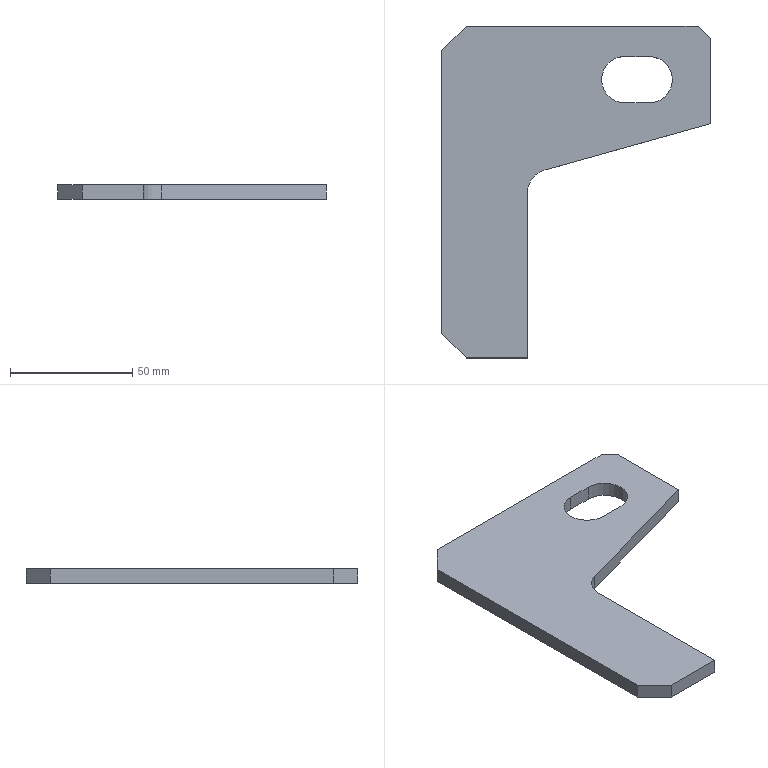Part | STEP file | 筋Plate-150×75-5 | 1 solid | 17 faces | box 110 x 136 x 6 mm | volume 47835 mm3 | plane 13 | cylinder 4 | commonest cylinder face diameters 19 x3 20 x1
STEP:
#1=CARTESIAN_POINT('',(0.,0.,0.));
#2=DIRECTION('',(0.,0.,1.));
#3=DIRECTION('',(1.,0.,0.));
#4=AXIS2_PLACEMENT_3D('',#1,#2,#3);
#5=CARTESIAN_POINT('',(20.,55.5,3.));
#6=VERTEX_POINT('',#5);
#7=CARTESIAN_POINT('',(20.,55.5,-3.));
#8=VERTEX_POINT('',#7);
#9=CARTESIAN_POINT('',(20.,55.5,-3.));
#10=DIRECTION('',(0.,0.,-1.));
#11=VECTOR('',#10,1.);
#12=LINE('',#9,#11);
#13=CARTESIAN_POINT('',(20.,46.,-3.));
#14=DIRECTION('',(0.,0.,-1.));
#15=DIRECTION('',(-1.,0.,0.));
#16=AXIS2_PLACEMENT_3D('',#13,#14,#15);
#17=CYLINDRICAL_SURFACE('',#16,9.5);
#18=CARTESIAN_POINT('',(1.571,0.));
#19=DIRECTION('',(0.,1.));
#20=VECTOR('',#19,1.);
#21=LINE('',#18,#20);
#22=(GEOMETRIC_REPRESENTATION_CONTEXT(2)PARAMETRIC_REPRESENTATION_CONTEXT()REPRESENTATION_CONTEXT('',''));
#23=DEFINITIONAL_REPRESENTATION('',(#21),#22);
#24=PCURVE('',#17,#23);
#25=CARTESIAN_POINT('',(20.,55.5,-3.));
#26=DIRECTION('',(0.,1.,0.));
#27=DIRECTION('',(0.,0.,1.));
#28=AXIS2_PLACEMENT_3D('',#25,#26,#27);
#29=PLANE('',#28);
#30=CARTESIAN_POINT('',(0.,0.));
#31=DIRECTION('',(-1.,0.));
#32=VECTOR('',#31,1.);
#33=LINE('',#30,#32);
#34=(GEOMETRIC_REPRESENTATION_CONTEXT(2)PARAMETRIC_REPRESENTATION_CONTEXT()REPRESENTATION_CONTEXT('',''));
#35=DEFINITIONAL_REPRESENTATION('',(#33),#34);
#36=PCURVE('',#29,#35);
#37=SURFACE_CURVE('',#12,(#24,#36),.PCURVE_S1.);
#38=EDGE_CURVE('',#6,#8,#37,.T.);
#39=ORIENTED_EDGE('',*,*,#38,.T.);
#40=CARTESIAN_POINT('',(10.5,46.,-3.));
#41=VERTEX_POINT('',#40);
#42=CARTESIAN_POINT('',(20.,46.,-3.));
#43=DIRECTION('',(0.,0.,-1.));
#44=DIRECTION('',(-1.,0.,0.));
#45=AXIS2_PLACEMENT_3D('',#42,#43,#44);
#46=CIRCLE('',#45,9.5);
#47=CARTESIAN_POINT('',(0.,0.));
#48=DIRECTION('',(1.,0.));
#49=VECTOR('',#48,1.);
#50=LINE('',#47,#49);
#51=(GEOMETRIC_REPRESENTATION_CONTEXT(2)PARAMETRIC_REPRESENTATION_CONTEXT()REPRESENTATION_CONTEXT('',''));
#52=DEFINITIONAL_REPRESENTATION('',(#50),#51);
#53=PCURVE('',#17,#52);
#54=CARTESIAN_POINT('',(0.,0.,-3.));
#55=DIRECTION('',(0.,0.,1.));
#56=DIRECTION('',(1.,0.,0.));
#57=AXIS2_PLACEMENT_3D('',#54,#55,#56);
#58=PLANE('',#57);
#59=CARTESIAN_POINT('',(10.5,46.));
#60=CARTESIAN_POINT('',(10.5,62.454));
#61=CARTESIAN_POINT('',(24.75,54.227));
#62=CARTESIAN_POINT('',(39.,46.));
#63=CARTESIAN_POINT('',(24.75,37.773));
#64=CARTESIAN_POINT('',(10.5,29.546));
#65=CARTESIAN_POINT('',(10.5,46.));
#66=(BOUNDED_CURVE()B_SPLINE_CURVE(2,(#59,#60,#61,#62,#63,#64,#65),.UNSPECIFIED.,.T.,.F.)B_SPLINE_CURVE_WITH_KNOTS((1,2,2,2,2,1),(-2.094,0.,2.094,4.189,6.283,8.378),.UNSPECIFIED.)CURVE()GEOMETRIC_REPRESENTATION_ITEM()RATIONAL_B_SPLINE_CURVE((1.,0.5,1.,0.5,1.,0.5,1.))REPRESENTATION_ITEM(''));
#67=(GEOMETRIC_REPRESENTATION_CONTEXT(2)PARAMETRIC_REPRESENTATION_CONTEXT()REPRESENTATION_CONTEXT('',''));
#68=DEFINITIONAL_REPRESENTATION('',(#66),#67);
#69=PCURVE('',#58,#68);
#70=SURFACE_CURVE('',#46,(#53,#69),.PCURVE_S1.);
#71=EDGE_CURVE('',#41,#8,#70,.T.);
#72=ORIENTED_EDGE('',*,*,#71,.F.);
#73=CARTESIAN_POINT('',(10.5,46.,3.));
#74=VERTEX_POINT('',#73);
#75=CARTESIAN_POINT('',(10.5,46.,-3.));
#76=DIRECTION('',(0.,0.,-1.));
#77=VECTOR('',#76,1.);
#78=LINE('',#75,#77);
#79=CARTESIAN_POINT('',(0.,0.));
#80=DIRECTION('',(0.,1.));
#81=VECTOR('',#80,1.);
#82=LINE('',#79,#81);
#83=(GEOMETRIC_REPRESENTATION_CONTEXT(2)PARAMETRIC_REPRESENTATION_CONTEXT()REPRESENTATION_CONTEXT('',''));
#84=DEFINITIONAL_REPRESENTATION('',(#82),#83);
#85=PCURVE('',#17,#84);
#86=CARTESIAN_POINT('',(20.,46.,-3.));
#87=DIRECTION('',(0.,0.,-1.));
#88=DIRECTION('',(-1.,0.,0.));
#89=AXIS2_PLACEMENT_3D('',#86,#87,#88);
#90=CYLINDRICAL_SURFACE('',#89,9.5);
#91=CARTESIAN_POINT('',(6.283,0.));
#92=DIRECTION('',(0.,1.));
#93=VECTOR('',#92,1.);
#94=LINE('',#91,#93);
#95=(GEOMETRIC_REPRESENTATION_CONTEXT(2)PARAMETRIC_REPRESENTATION_CONTEXT()REPRESENTATION_CONTEXT('',''));
#96=DEFINITIONAL_REPRESENTATION('',(#94),#95);
#97=PCURVE('',#90,#96);
#98=SURFACE_CURVE('',#78,(#85,#97),.PCURVE_S1.);
#99=EDGE_CURVE('',#74,#41,#98,.T.);
#100=ORIENTED_EDGE('',*,*,#99,.F.);
#101=CARTESIAN_POINT('',(20.,46.,3.));
#102=DIRECTION('',(0.,0.,1.));
#103=DIRECTION('',(1.,0.,0.));
#104=AXIS2_PLACEMENT_3D('',#101,#102,#103);
#105=CIRCLE('',#104,9.5);
#106=CARTESIAN_POINT('',(3.142,-6.));
#107=DIRECTION('',(-1.,0.));
#108=VECTOR('',#107,1.);
#109=LINE('',#106,#108);
#110=(GEOMETRIC_REPRESENTATION_CONTEXT(2)PARAMETRIC_REPRESENTATION_CONTEXT()REPRESENTATION_CONTEXT('',''));
#111=DEFINITIONAL_REPRESENTATION('',(#109),#110);
#112=PCURVE('',#17,#111);
#113=CARTESIAN_POINT('',(0.,0.,3.));
#114=DIRECTION('',(0.,0.,1.));
#115=DIRECTION('',(1.,0.,0.));
#116=AXIS2_PLACEMENT_3D('',#113,#114,#115);
#117=PLANE('',#116);
#118=CARTESIAN_POINT('',(20.,46.));
#119=DIRECTION('',(1.,0.));
#120=AXIS2_PLACEMENT_2D('',#118,#119);
#121=CIRCLE('',#120,9.5);
#122=(GEOMETRIC_REPRESENTATION_CONTEXT(2)PARAMETRIC_REPRESENTATION_CONTEXT()REPRESENTATION_CONTEXT('',''));
#123=DEFINITIONAL_REPRESENTATION('',(#121),#122);
#124=PCURVE('',#117,#123);
#125=SURFACE_CURVE('',#105,(#112,#124),.PCURVE_S1.);
#126=EDGE_CURVE('',#6,#74,#125,.T.);
#127=ORIENTED_EDGE('',*,*,#126,.F.);
#128=EDGE_LOOP('',(#39,#72,#100,#127));
#129=FACE_BOUND('',#128,.F.);
#130=ADVANCED_FACE('',(#129),#17,.F.);
#131=CARTESIAN_POINT('',(-45.,68.,-3.));
#132=VERTEX_POINT('',#131);
#133=CARTESIAN_POINT('',(50.,68.,-3.));
#134=VERTEX_POINT('',#133);
#135=CARTESIAN_POINT('',(0.,68.,-3.));
#136=DIRECTION('',(1.,0.,0.));
#137=VECTOR('',#136,1.);
#138=LINE('',#135,#137);
#139=CARTESIAN_POINT('',(0.,68.));
#140=DIRECTION('',(1.,0.));
#141=VECTOR('',#140,1.);
#142=LINE('',#139,#141);
#143=(GEOMETRIC_REPRESENTATION_CONTEXT(2)PARAMETRIC_REPRESENTATION_CONTEXT()REPRESENTATION_CONTEXT('',''));
#144=DEFINITIONAL_REPRESENTATION('',(#142),#143);
#145=PCURVE('',#58,#144);
#146=CARTESIAN_POINT('',(0.,68.,3.));
#147=DIRECTION('',(0.,1.,0.));
#148=DIRECTION('',(0.,0.,1.));
#149=AXIS2_PLACEMENT_3D('',#146,#147,#148);
#150=PLANE('',#149);
#151=CARTESIAN_POINT('',(-6.,0.));
#152=DIRECTION('',(0.,1.));
#153=VECTOR('',#152,1.);
#154=LINE('',#151,#153);
#155=(GEOMETRIC_REPRESENTATION_CONTEXT(2)PARAMETRIC_REPRESENTATION_CONTEXT()REPRESENTATION_CONTEXT('',''));
#156=DEFINITIONAL_REPRESENTATION('',(#154),#155);
#157=PCURVE('',#150,#156);
#158=SURFACE_CURVE('',#138,(#145,#157),.PCURVE_S1.);
#159=EDGE_CURVE('',#132,#134,#158,.T.);
#160=ORIENTED_EDGE('',*,*,#159,.T.);
#161=CARTESIAN_POINT('',(55.,63.,-3.));
#162=VERTEX_POINT('',#161);
#163=CARTESIAN_POINT('',(50.,68.,-3.));
#164=DIRECTION('',(0.7071,-0.7071,0.));
#165=VECTOR('',#164,1.);
#166=LINE('',#163,#165);
#167=CARTESIAN_POINT('',(50.,68.));
#168=DIRECTION('',(0.7071,-0.7071));
#169=VECTOR('',#168,1.);
#170=LINE('',#167,#169);
#171=(GEOMETRIC_REPRESENTATION_CONTEXT(2)PARAMETRIC_REPRESENTATION_CONTEXT()REPRESENTATION_CONTEXT('',''));
#172=DEFINITIONAL_REPRESENTATION('',(#170),#171);
#173=PCURVE('',#58,#172);
#174=CARTESIAN_POINT('',(50.,68.,3.));
#175=DIRECTION('',(-0.7071,-0.7071,0.));
#176=DIRECTION('',(0.,0.,-1.));
#177=AXIS2_PLACEMENT_3D('',#174,#175,#176);
#178=PLANE('',#177);
#179=CARTESIAN_POINT('',(6.,0.));
#180=DIRECTION('',(0.,1.));
#181=VECTOR('',#180,1.);
#182=LINE('',#179,#181);
#183=(GEOMETRIC_REPRESENTATION_CONTEXT(2)PARAMETRIC_REPRESENTATION_CONTEXT()REPRESENTATION_CONTEXT('',''));
#184=DEFINITIONAL_REPRESENTATION('',(#182),#183);
#185=PCURVE('',#178,#184);
#186=SURFACE_CURVE('',#166,(#173,#185),.PCURVE_S1.);
#187=EDGE_CURVE('',#134,#162,#186,.T.);
#188=ORIENTED_EDGE('',*,*,#187,.T.);
#189=CARTESIAN_POINT('',(55.,28.,-3.));
#190=VERTEX_POINT('',#189);
#191=CARTESIAN_POINT('',(55.,0.,-3.));
#192=DIRECTION('',(0.,-1.,0.));
#193=VECTOR('',#192,1.);
#194=LINE('',#191,#193);
#195=CARTESIAN_POINT('',(55.,0.));
#196=DIRECTION('',(0.,-1.));
#197=VECTOR('',#196,1.);
#198=LINE('',#195,#197);
#199=(GEOMETRIC_REPRESENTATION_CONTEXT(2)PARAMETRIC_REPRESENTATION_CONTEXT()REPRESENTATION_CONTEXT('',''));
#200=DEFINITIONAL_REPRESENTATION('',(#198),#199);
#201=PCURVE('',#58,#200);
#202=CARTESIAN_POINT('',(55.,0.,3.));
#203=DIRECTION('',(1.,0.,0.));
#204=DIRECTION('',(0.,1.,0.));
#205=AXIS2_PLACEMENT_3D('',#202,#203,#204);
#206=PLANE('',#205);
#207=CARTESIAN_POINT('',(0.,-6.));
#208=DIRECTION('',(-1.,0.));
#209=VECTOR('',#208,1.);
#210=LINE('',#207,#209);
#211=(GEOMETRIC_REPRESENTATION_CONTEXT(2)PARAMETRIC_REPRESENTATION_CONTEXT()REPRESENTATION_CONTEXT('',''));
#212=DEFINITIONAL_REPRESENTATION('',(#210),#211);
#213=PCURVE('',#206,#212);
#214=SURFACE_CURVE('',#194,(#201,#213),.PCURVE_S1.);
#215=EDGE_CURVE('',#162,#190,#214,.T.);
#216=ORIENTED_EDGE('',*,*,#215,.T.);
#217=CARTESIAN_POINT('',(-12.696,9.045,-3.));
#218=VERTEX_POINT('',#217);
#219=CARTESIAN_POINT('',(55.,28.,-3.));
#220=DIRECTION('',(-0.963,-0.2696,0.));
#221=VECTOR('',#220,1.);
#222=LINE('',#219,#221);
#223=CARTESIAN_POINT('',(55.,28.));
#224=DIRECTION('',(-0.963,-0.2696));
#225=VECTOR('',#224,1.);
#226=LINE('',#223,#225);
#227=(GEOMETRIC_REPRESENTATION_CONTEXT(2)PARAMETRIC_REPRESENTATION_CONTEXT()REPRESENTATION_CONTEXT('',''));
#228=DEFINITIONAL_REPRESENTATION('',(#226),#227);
#229=PCURVE('',#58,#228);
#230=CARTESIAN_POINT('',(55.,28.,-3.));
#231=DIRECTION('',(-0.2696,0.963,0.));
#232=DIRECTION('',(-0.963,-0.2696,0.));
#233=AXIS2_PLACEMENT_3D('',#230,#231,#232);
#234=PLANE('',#233);
#235=CARTESIAN_POINT('',(0.,0.));
#236=DIRECTION('',(1.,0.));
#237=VECTOR('',#236,1.);
#238=LINE('',#235,#237);
#239=(GEOMETRIC_REPRESENTATION_CONTEXT(2)PARAMETRIC_REPRESENTATION_CONTEXT()REPRESENTATION_CONTEXT('',''));
#240=DEFINITIONAL_REPRESENTATION('',(#238),#239);
#241=PCURVE('',#234,#240);
#242=SURFACE_CURVE('',#222,(#229,#241),.PCURVE_S1.);
#243=EDGE_CURVE('',#190,#218,#242,.T.);
#244=ORIENTED_EDGE('',*,*,#243,.T.);
#245=CARTESIAN_POINT('',(-20.,-0.5846,-3.));
#246=VERTEX_POINT('',#245);
#247=CARTESIAN_POINT('',(-10.,-0.5846,-3.));
#248=DIRECTION('',(0.,0.,1.));
#249=DIRECTION('',(1.,0.,0.));
#250=AXIS2_PLACEMENT_3D('',#247,#248,#249);
#251=CIRCLE('',#250,10.);
#252=CARTESIAN_POINT('',(-10.,-0.5846));
#253=DIRECTION('',(1.,0.));
#254=AXIS2_PLACEMENT_2D('',#252,#253);
#255=CIRCLE('',#254,10.);
#256=(GEOMETRIC_REPRESENTATION_CONTEXT(2)PARAMETRIC_REPRESENTATION_CONTEXT()REPRESENTATION_CONTEXT('',''));
#257=DEFINITIONAL_REPRESENTATION('',(#255),#256);
#258=PCURVE('',#58,#257);
#259=CARTESIAN_POINT('',(-10.,-0.5846,-3.));
#260=DIRECTION('',(0.,0.,-1.));
#261=DIRECTION('',(-1.,0.,0.));
#262=AXIS2_PLACEMENT_3D('',#259,#260,#261);
#263=CYLINDRICAL_SURFACE('',#262,10.);
#264=CARTESIAN_POINT('',(3.142,0.));
#265=DIRECTION('',(-1.,0.));
#266=VECTOR('',#265,1.);
#267=LINE('',#264,#266);
#268=(GEOMETRIC_REPRESENTATION_CONTEXT(2)PARAMETRIC_REPRESENTATION_CONTEXT()REPRESENTATION_CONTEXT('',''));
#269=DEFINITIONAL_REPRESENTATION('',(#267),#268);
#270=PCURVE('',#263,#269);
#271=SURFACE_CURVE('',#251,(#258,#270),.PCURVE_S1.);
#272=EDGE_CURVE('',#218,#246,#271,.T.);
#273=ORIENTED_EDGE('',*,*,#272,.T.);
#274=CARTESIAN_POINT('',(-20.,-68.,-3.));
#275=VERTEX_POINT('',#274);
#276=CARTESIAN_POINT('',(-20.,-68.,-3.));
#277=DIRECTION('',(0.,-1.,0.));
#278=VECTOR('',#277,1.);
#279=LINE('',#276,#278);
#280=CARTESIAN_POINT('',(-20.,-68.));
#281=DIRECTION('',(0.,-1.));
#282=VECTOR('',#281,1.);
#283=LINE('',#280,#282);
#284=(GEOMETRIC_REPRESENTATION_CONTEXT(2)PARAMETRIC_REPRESENTATION_CONTEXT()REPRESENTATION_CONTEXT('',''));
#285=DEFINITIONAL_REPRESENTATION('',(#283),#284);
#286=PCURVE('',#58,#285);
#287=CARTESIAN_POINT('',(-20.,-68.,-3.));
#288=DIRECTION('',(-1.,0.,0.));
#289=DIRECTION('',(0.,0.,1.));
#290=AXIS2_PLACEMENT_3D('',#287,#288,#289);
#291=PLANE('',#290);
#292=CARTESIAN_POINT('',(0.,0.));
#293=DIRECTION('',(0.,-1.));
#294=VECTOR('',#293,1.);
#295=LINE('',#292,#294);
#296=(GEOMETRIC_REPRESENTATION_CONTEXT(2)PARAMETRIC_REPRESENTATION_CONTEXT()REPRESENTATION_CONTEXT('',''));
#297=DEFINITIONAL_REPRESENTATION('',(#295),#296);
#298=PCURVE('',#291,#297);
#299=SURFACE_CURVE('',#279,(#286,#298),.PCURVE_S1.);
#300=EDGE_CURVE('',#246,#275,#299,.T.);
#301=ORIENTED_EDGE('',*,*,#300,.T.);
#302=CARTESIAN_POINT('',(-45.,-68.,-3.));
#303=VERTEX_POINT('',#302);
#304=CARTESIAN_POINT('',(0.,-68.,-3.));
#305=DIRECTION('',(1.,0.,0.));
#306=VECTOR('',#305,1.);
#307=LINE('',#304,#306);
#308=CARTESIAN_POINT('',(0.,-68.));
#309=DIRECTION('',(1.,0.));
#310=VECTOR('',#309,1.);
#311=LINE('',#308,#310);
#312=(GEOMETRIC_REPRESENTATION_CONTEXT(2)PARAMETRIC_REPRESENTATION_CONTEXT()REPRESENTATION_CONTEXT('',''));
#313=DEFINITIONAL_REPRESENTATION('',(#311),#312);
#314=PCURVE('',#58,#313);
#315=CARTESIAN_POINT('',(0.,-68.,3.));
#316=DIRECTION('',(0.,1.,0.));
#317=DIRECTION('',(0.,0.,1.));
#318=AXIS2_PLACEMENT_3D('',#315,#316,#317);
#319=PLANE('',#318);
#320=CARTESIAN_POINT('',(-6.,0.));
#321=DIRECTION('',(0.,1.));
#322=VECTOR('',#321,1.);
#323=LINE('',#320,#322);
#324=(GEOMETRIC_REPRESENTATION_CONTEXT(2)PARAMETRIC_REPRESENTATION_CONTEXT()REPRESENTATION_CONTEXT('',''));
#325=DEFINITIONAL_REPRESENTATION('',(#323),#324);
#326=PCURVE('',#319,#325);
#327=SURFACE_CURVE('',#307,(#314,#326),.PCURVE_S1.);
#328=EDGE_CURVE('',#303,#275,#327,.T.);
#329=ORIENTED_EDGE('',*,*,#328,.F.);
#330=CARTESIAN_POINT('',(-55.,-58.,-3.));
#331=VERTEX_POINT('',#330);
#332=CARTESIAN_POINT('',(-45.,-68.,-3.));
#333=DIRECTION('',(-0.7071,0.7071,0.));
#334=VECTOR('',#333,1.);
#335=LINE('',#332,#334);
#336=CARTESIAN_POINT('',(-45.,-68.));
#337=DIRECTION('',(-0.7071,0.7071));
#338=VECTOR('',#337,1.);
#339=LINE('',#336,#338);
#340=(GEOMETRIC_REPRESENTATION_CONTEXT(2)PARAMETRIC_REPRESENTATION_CONTEXT()REPRESENTATION_CONTEXT('',''));
#341=DEFINITIONAL_REPRESENTATION('',(#339),#340);
#342=PCURVE('',#58,#341);
#343=CARTESIAN_POINT('',(-45.,-68.,3.));
#344=DIRECTION('',(0.7071,0.7071,0.));
#345=DIRECTION('',(0.,0.,-1.));
#346=AXIS2_PLACEMENT_3D('',#343,#344,#345);
#347=PLANE('',#346);
#348=CARTESIAN_POINT('',(6.,0.));
#349=DIRECTION('',(0.,1.));
#350=VECTOR('',#349,1.);
#351=LINE('',#348,#350);
#352=(GEOMETRIC_REPRESENTATION_CONTEXT(2)PARAMETRIC_REPRESENTATION_CONTEXT()REPRESENTATION_CONTEXT('',''));
#353=DEFINITIONAL_REPRESENTATION('',(#351),#352);
#354=PCURVE('',#347,#353);
#355=SURFACE_CURVE('',#335,(#342,#354),.PCURVE_S1.);
#356=EDGE_CURVE('',#303,#331,#355,.T.);
#357=ORIENTED_EDGE('',*,*,#356,.T.);
#358=CARTESIAN_POINT('',(-55.,58.,-3.));
#359=VERTEX_POINT('',#358);
#360=CARTESIAN_POINT('',(-55.,0.,-3.));
#361=DIRECTION('',(0.,-1.,0.));
#362=VECTOR('',#361,1.);
#363=LINE('',#360,#362);
#364=CARTESIAN_POINT('',(-55.,0.));
#365=DIRECTION('',(0.,-1.));
#366=VECTOR('',#365,1.);
#367=LINE('',#364,#366);
#368=(GEOMETRIC_REPRESENTATION_CONTEXT(2)PARAMETRIC_REPRESENTATION_CONTEXT()REPRESENTATION_CONTEXT('',''));
#369=DEFINITIONAL_REPRESENTATION('',(#367),#368);
#370=PCURVE('',#58,#369);
#371=CARTESIAN_POINT('',(-55.,0.,3.));
#372=DIRECTION('',(1.,0.,0.));
#373=DIRECTION('',(0.,1.,0.));
#374=AXIS2_PLACEMENT_3D('',#371,#372,#373);
#375=PLANE('',#374);
#376=CARTESIAN_POINT('',(0.,-6.));
#377=DIRECTION('',(-1.,0.));
#378=VECTOR('',#377,1.);
#379=LINE('',#376,#378);
#380=(GEOMETRIC_REPRESENTATION_CONTEXT(2)PARAMETRIC_REPRESENTATION_CONTEXT()REPRESENTATION_CONTEXT('',''));
#381=DEFINITIONAL_REPRESENTATION('',(#379),#380);
#382=PCURVE('',#375,#381);
#383=SURFACE_CURVE('',#363,(#370,#382),.PCURVE_S1.);
#384=EDGE_CURVE('',#359,#331,#383,.T.);
#385=ORIENTED_EDGE('',*,*,#384,.F.);
#386=CARTESIAN_POINT('',(-55.,58.,-3.));
#387=DIRECTION('',(0.7071,0.7071,0.));
#388=VECTOR('',#387,1.);
#389=LINE('',#386,#388);
#390=CARTESIAN_POINT('',(-55.,58.));
#391=DIRECTION('',(0.7071,0.7071));
#392=VECTOR('',#391,1.);
#393=LINE('',#390,#392);
#394=(GEOMETRIC_REPRESENTATION_CONTEXT(2)PARAMETRIC_REPRESENTATION_CONTEXT()REPRESENTATION_CONTEXT('',''));
#395=DEFINITIONAL_REPRESENTATION('',(#393),#394);
#396=PCURVE('',#58,#395);
#397=CARTESIAN_POINT('',(-55.,58.,3.));
#398=DIRECTION('',(-0.7071,0.7071,0.));
#399=DIRECTION('',(0.,0.,1.));
#400=AXIS2_PLACEMENT_3D('',#397,#398,#399);
#401=PLANE('',#400);
#402=CARTESIAN_POINT('',(-6.,0.));
#403=DIRECTION('',(0.,1.));
#404=VECTOR('',#403,1.);
#405=LINE('',#402,#404);
#406=(GEOMETRIC_REPRESENTATION_CONTEXT(2)PARAMETRIC_REPRESENTATION_CONTEXT()REPRESENTATION_CONTEXT('',''));
#407=DEFINITIONAL_REPRESENTATION('',(#405),#406);
#408=PCURVE('',#401,#407);
#409=SURFACE_CURVE('',#389,(#396,#408),.PCURVE_S1.);
#410=EDGE_CURVE('',#359,#132,#409,.T.);
#411=ORIENTED_EDGE('',*,*,#410,.T.);
#412=EDGE_LOOP('',(#160,#188,#216,#244,#273,#301,#329,#357,#385,#411));
#413=FACE_BOUND('',#412,.T.);
#414=CARTESIAN_POINT('',(30.,55.5,-3.));
#415=VERTEX_POINT('',#414);
#416=CARTESIAN_POINT('',(30.,36.5,-3.));
#417=VERTEX_POINT('',#416);
#418=CARTESIAN_POINT('',(30.,46.,-3.));
#419=DIRECTION('',(0.,0.,-1.));
#420=DIRECTION('',(-1.,0.,0.));
#421=AXIS2_PLACEMENT_3D('',#418,#419,#420);
#422=CIRCLE('',#421,9.5);
#423=CARTESIAN_POINT('',(20.5,46.));
#424=CARTESIAN_POINT('',(20.5,62.454));
#425=CARTESIAN_POINT('',(34.75,54.227));
#426=CARTESIAN_POINT('',(49.,46.));
#427=CARTESIAN_POINT('',(34.75,37.773));
#428=CARTESIAN_POINT('',(20.5,29.546));
#429=CARTESIAN_POINT('',(20.5,46.));
#430=(BOUNDED_CURVE()B_SPLINE_CURVE(2,(#423,#424,#425,#426,#427,#428,#429),.UNSPECIFIED.,.T.,.F.)B_SPLINE_CURVE_WITH_KNOTS((1,2,2,2,2,1),(-2.094,0.,2.094,4.189,6.283,8.378),.UNSPECIFIED.)CURVE()GEOMETRIC_REPRESENTATION_ITEM()RATIONAL_B_SPLINE_CURVE((1.,0.5,1.,0.5,1.,0.5,1.))REPRESENTATION_ITEM(''));
#431=(GEOMETRIC_REPRESENTATION_CONTEXT(2)PARAMETRIC_REPRESENTATION_CONTEXT()REPRESENTATION_CONTEXT('',''));
#432=DEFINITIONAL_REPRESENTATION('',(#430),#431);
#433=PCURVE('',#58,#432);
#434=CARTESIAN_POINT('',(30.,46.,-3.));
#435=DIRECTION('',(0.,0.,-1.));
#436=DIRECTION('',(-1.,0.,0.));
#437=AXIS2_PLACEMENT_3D('',#434,#435,#436);
#438=CYLINDRICAL_SURFACE('',#437,9.5);
#439=CARTESIAN_POINT('',(0.,0.));
#440=DIRECTION('',(1.,0.));
#441=VECTOR('',#440,1.);
#442=LINE('',#439,#441);
#443=(GEOMETRIC_REPRESENTATION_CONTEXT(2)PARAMETRIC_REPRESENTATION_CONTEXT()REPRESENTATION_CONTEXT('',''));
#444=DEFINITIONAL_REPRESENTATION('',(#442),#443);
#445=PCURVE('',#438,#444);
#446=SURFACE_CURVE('',#422,(#433,#445),.PCURVE_S1.);
#447=EDGE_CURVE('',#415,#417,#446,.T.);
#448=ORIENTED_EDGE('',*,*,#447,.F.);
#449=CARTESIAN_POINT('',(20.,55.5,-3.));
#450=DIRECTION('',(1.,0.,0.));
#451=VECTOR('',#450,1.);
#452=LINE('',#449,#451);
#453=CARTESIAN_POINT('',(20.,55.5));
#454=DIRECTION('',(1.,0.));
#455=VECTOR('',#454,1.);
#456=LINE('',#453,#455);
#457=(GEOMETRIC_REPRESENTATION_CONTEXT(2)PARAMETRIC_REPRESENTATION_CONTEXT()REPRESENTATION_CONTEXT('',''));
#458=DEFINITIONAL_REPRESENTATION('',(#456),#457);
#459=PCURVE('',#58,#458);
#460=CARTESIAN_POINT('',(0.,0.));
#461=DIRECTION('',(0.,1.));
#462=VECTOR('',#461,1.);
#463=LINE('',#460,#462);
#464=(GEOMETRIC_REPRESENTATION_CONTEXT(2)PARAMETRIC_REPRESENTATION_CONTEXT()REPRESENTATION_CONTEXT('',''));
#465=DEFINITIONAL_REPRESENTATION('',(#463),#464);
#466=PCURVE('',#29,#465);
#467=SURFACE_CURVE('',#452,(#459,#466),.PCURVE_S1.);
#468=EDGE_CURVE('',#8,#415,#467,.T.);
#469=ORIENTED_EDGE('',*,*,#468,.F.);
#470=ORIENTED_EDGE('',*,*,#71,.F.);
#471=CARTESIAN_POINT('',(20.,36.5,-3.));
#472=VERTEX_POINT('',#471);
#473=CARTESIAN_POINT('',(20.,46.,-3.));
#474=DIRECTION('',(0.,0.,-1.));
#475=DIRECTION('',(-1.,0.,0.));
#476=AXIS2_PLACEMENT_3D('',#473,#474,#475);
#477=CIRCLE('',#476,9.5);
#478=CARTESIAN_POINT('',(10.5,46.));
#479=CARTESIAN_POINT('',(10.5,62.454));
#480=CARTESIAN_POINT('',(24.75,54.227));
#481=CARTESIAN_POINT('',(39.,46.));
#482=CARTESIAN_POINT('',(24.75,37.773));
#483=CARTESIAN_POINT('',(10.5,29.546));
#484=CARTESIAN_POINT('',(10.5,46.));
#485=(BOUNDED_CURVE()B_SPLINE_CURVE(2,(#478,#479,#480,#481,#482,#483,#484),.UNSPECIFIED.,.T.,.F.)B_SPLINE_CURVE_WITH_KNOTS((1,2,2,2,2,1),(-2.094,0.,2.094,4.189,6.283,8.378),.UNSPECIFIED.)CURVE()GEOMETRIC_REPRESENTATION_ITEM()RATIONAL_B_SPLINE_CURVE((1.,0.5,1.,0.5,1.,0.5,1.))REPRESENTATION_ITEM(''));
#486=(GEOMETRIC_REPRESENTATION_CONTEXT(2)PARAMETRIC_REPRESENTATION_CONTEXT()REPRESENTATION_CONTEXT('',''));
#487=DEFINITIONAL_REPRESENTATION('',(#485),#486);
#488=PCURVE('',#58,#487);
#489=CARTESIAN_POINT('',(0.,0.));
#490=DIRECTION('',(1.,0.));
#491=VECTOR('',#490,1.);
#492=LINE('',#489,#491);
#493=(GEOMETRIC_REPRESENTATION_CONTEXT(2)PARAMETRIC_REPRESENTATION_CONTEXT()REPRESENTATION_CONTEXT('',''));
#494=DEFINITIONAL_REPRESENTATION('',(#492),#493);
#495=PCURVE('',#90,#494);
#496=SURFACE_CURVE('',#477,(#488,#495),.PCURVE_S1.);
#497=EDGE_CURVE('',#472,#41,#496,.T.);
#498=ORIENTED_EDGE('',*,*,#497,.F.);
#499=CARTESIAN_POINT('',(20.,36.5,-3.));
#500=DIRECTION('',(1.,0.,0.));
#501=VECTOR('',#500,1.);
#502=LINE('',#499,#501);
#503=CARTESIAN_POINT('',(20.,36.5));
#504=DIRECTION('',(1.,0.));
#505=VECTOR('',#504,1.);
#506=LINE('',#503,#505);
#507=(GEOMETRIC_REPRESENTATION_CONTEXT(2)PARAMETRIC_REPRESENTATION_CONTEXT()REPRESENTATION_CONTEXT('',''));
#508=DEFINITIONAL_REPRESENTATION('',(#506),#507);
#509=PCURVE('',#58,#508);
#510=CARTESIAN_POINT('',(20.,36.5,-3.));
#511=DIRECTION('',(0.,-1.,0.));
#512=DIRECTION('',(0.,0.,-1.));
#513=AXIS2_PLACEMENT_3D('',#510,#511,#512);
#514=PLANE('',#513);
#515=CARTESIAN_POINT('',(0.,0.));
#516=DIRECTION('',(0.,1.));
#517=VECTOR('',#516,1.);
#518=LINE('',#515,#517);
#519=(GEOMETRIC_REPRESENTATION_CONTEXT(2)PARAMETRIC_REPRESENTATION_CONTEXT()REPRESENTATION_CONTEXT('',''));
#520=DEFINITIONAL_REPRESENTATION('',(#518),#519);
#521=PCURVE('',#514,#520);
#522=SURFACE_CURVE('',#502,(#509,#521),.PCURVE_S1.);
#523=EDGE_CURVE('',#472,#417,#522,.T.);
#524=ORIENTED_EDGE('',*,*,#523,.T.);
#525=EDGE_LOOP('',(#448,#469,#470,#498,#524));
#526=FACE_BOUND('',#525,.T.);
#527=ADVANCED_FACE('',(#413,#526),#58,.F.);
#528=ORIENTED_EDGE('',*,*,#215,.F.);
#529=CARTESIAN_POINT('',(55.,63.,3.));
#530=VERTEX_POINT('',#529);
#531=CARTESIAN_POINT('',(55.,63.,3.));
#532=DIRECTION('',(0.,0.,1.));
#533=VECTOR('',#532,1.);
#534=LINE('',#531,#533);
#535=CARTESIAN_POINT('',(63.,0.));
#536=DIRECTION('',(0.,1.));
#537=VECTOR('',#536,1.);
#538=LINE('',#535,#537);
#539=(GEOMETRIC_REPRESENTATION_CONTEXT(2)PARAMETRIC_REPRESENTATION_CONTEXT()REPRESENTATION_CONTEXT('',''));
#540=DEFINITIONAL_REPRESENTATION('',(#538),#539);
#541=PCURVE('',#206,#540);
#542=CARTESIAN_POINT('',(0.,7.071));
#543=DIRECTION('',(-1.,0.));
#544=VECTOR('',#543,1.);
#545=LINE('',#542,#544);
#546=(GEOMETRIC_REPRESENTATION_CONTEXT(2)PARAMETRIC_REPRESENTATION_CONTEXT()REPRESENTATION_CONTEXT('',''));
#547=DEFINITIONAL_REPRESENTATION('',(#545),#546);
#548=PCURVE('',#178,#547);
#549=SURFACE_CURVE('',#534,(#541,#548),.PCURVE_S1.);
#550=EDGE_CURVE('',#162,#530,#549,.T.);
#551=ORIENTED_EDGE('',*,*,#550,.T.);
#552=CARTESIAN_POINT('',(55.,28.,3.));
#553=VERTEX_POINT('',#552);
#554=CARTESIAN_POINT('',(55.,0.,3.));
#555=DIRECTION('',(0.,-1.,0.));
#556=VECTOR('',#555,1.);
#557=LINE('',#554,#556);
#558=CARTESIAN_POINT('',(0.,0.));
#559=DIRECTION('',(-1.,0.));
#560=VECTOR('',#559,1.);
#561=LINE('',#558,#560);
#562=(GEOMETRIC_REPRESENTATION_CONTEXT(2)PARAMETRIC_REPRESENTATION_CONTEXT()REPRESENTATION_CONTEXT('',''));
#563=DEFINITIONAL_REPRESENTATION('',(#561),#562);
#564=PCURVE('',#206,#563);
#565=CARTESIAN_POINT('',(55.,0.));
#566=DIRECTION('',(0.,-1.));
#567=VECTOR('',#566,1.);
#568=LINE('',#565,#567);
#569=(GEOMETRIC_REPRESENTATION_CONTEXT(2)PARAMETRIC_REPRESENTATION_CONTEXT()REPRESENTATION_CONTEXT('',''));
#570=DEFINITIONAL_REPRESENTATION('',(#568),#569);
#571=PCURVE('',#117,#570);
#572=SURFACE_CURVE('',#557,(#564,#571),.PCURVE_S1.);
#573=EDGE_CURVE('',#530,#553,#572,.T.);
#574=ORIENTED_EDGE('',*,*,#573,.T.);
#575=CARTESIAN_POINT('',(55.,28.,-3.));
#576=DIRECTION('',(0.,0.,1.));
#577=VECTOR('',#576,1.);
#578=LINE('',#575,#577);
#579=CARTESIAN_POINT('',(28.,-6.));
#580=DIRECTION('',(0.,1.));
#581=VECTOR('',#580,1.);
#582=LINE('',#579,#581);
#583=(GEOMETRIC_REPRESENTATION_CONTEXT(2)PARAMETRIC_REPRESENTATION_CONTEXT()REPRESENTATION_CONTEXT('',''));
#584=DEFINITIONAL_REPRESENTATION('',(#582),#583);
#585=PCURVE('',#206,#584);
#586=CARTESIAN_POINT('',(0.,0.));
#587=DIRECTION('',(0.,1.));
#588=VECTOR('',#587,1.);
#589=LINE('',#586,#588);
#590=(GEOMETRIC_REPRESENTATION_CONTEXT(2)PARAMETRIC_REPRESENTATION_CONTEXT()REPRESENTATION_CONTEXT('',''));
#591=DEFINITIONAL_REPRESENTATION('',(#589),#590);
#592=PCURVE('',#234,#591);
#593=SURFACE_CURVE('',#578,(#585,#592),.PCURVE_S1.);
#594=EDGE_CURVE('',#190,#553,#593,.T.);
#595=ORIENTED_EDGE('',*,*,#594,.F.);
#596=EDGE_LOOP('',(#528,#551,#574,#595));
#597=FACE_BOUND('',#596,.T.);
#598=ADVANCED_FACE('',(#597),#206,.T.);
#599=CARTESIAN_POINT('',(-45.,68.,3.));
#600=VERTEX_POINT('',#599);
#601=CARTESIAN_POINT('',(50.,68.,3.));
#602=VERTEX_POINT('',#601);
#603=CARTESIAN_POINT('',(0.,68.,3.));
#604=DIRECTION('',(1.,0.,0.));
#605=VECTOR('',#604,1.);
#606=LINE('',#603,#605);
#607=CARTESIAN_POINT('',(0.,0.));
#608=DIRECTION('',(0.,1.));
#609=VECTOR('',#608,1.);
#610=LINE('',#607,#609);
#611=(GEOMETRIC_REPRESENTATION_CONTEXT(2)PARAMETRIC_REPRESENTATION_CONTEXT()REPRESENTATION_CONTEXT('',''));
#612=DEFINITIONAL_REPRESENTATION('',(#610),#611);
#613=PCURVE('',#150,#612);
#614=CARTESIAN_POINT('',(0.,68.));
#615=DIRECTION('',(1.,0.));
#616=VECTOR('',#615,1.);
#617=LINE('',#614,#616);
#618=(GEOMETRIC_REPRESENTATION_CONTEXT(2)PARAMETRIC_REPRESENTATION_CONTEXT()REPRESENTATION_CONTEXT('',''));
#619=DEFINITIONAL_REPRESENTATION('',(#617),#618);
#620=PCURVE('',#117,#619);
#621=SURFACE_CURVE('',#606,(#613,#620),.PCURVE_S1.);
#622=EDGE_CURVE('',#600,#602,#621,.T.);
#623=ORIENTED_EDGE('',*,*,#622,.T.);
#624=CARTESIAN_POINT('',(50.,68.,3.));
#625=DIRECTION('',(0.,0.,-1.));
#626=VECTOR('',#625,1.);
#627=LINE('',#624,#626);
#628=CARTESIAN_POINT('',(0.,50.));
#629=DIRECTION('',(-1.,0.));
#630=VECTOR('',#629,1.);
#631=LINE('',#628,#630);
#632=(GEOMETRIC_REPRESENTATION_CONTEXT(2)PARAMETRIC_REPRESENTATION_CONTEXT()REPRESENTATION_CONTEXT('',''));
#633=DEFINITIONAL_REPRESENTATION('',(#631),#632);
#634=PCURVE('',#150,#633);
#635=CARTESIAN_POINT('',(0.,0.));
#636=DIRECTION('',(1.,0.));
#637=VECTOR('',#636,1.);
#638=LINE('',#635,#637);
#639=(GEOMETRIC_REPRESENTATION_CONTEXT(2)PARAMETRIC_REPRESENTATION_CONTEXT()REPRESENTATION_CONTEXT('',''));
#640=DEFINITIONAL_REPRESENTATION('',(#638),#639);
#641=PCURVE('',#178,#640);
#642=SURFACE_CURVE('',#627,(#634,#641),.PCURVE_S1.);
#643=EDGE_CURVE('',#602,#134,#642,.T.);
#644=ORIENTED_EDGE('',*,*,#643,.T.);
#645=ORIENTED_EDGE('',*,*,#159,.F.);
#646=CARTESIAN_POINT('',(-45.,68.,3.));
#647=DIRECTION('',(0.,0.,1.));
#648=VECTOR('',#647,1.);
#649=LINE('',#646,#648);
#650=CARTESIAN_POINT('',(0.,-45.));
#651=DIRECTION('',(1.,0.));
#652=VECTOR('',#651,1.);
#653=LINE('',#650,#652);
#654=(GEOMETRIC_REPRESENTATION_CONTEXT(2)PARAMETRIC_REPRESENTATION_CONTEXT()REPRESENTATION_CONTEXT('',''));
#655=DEFINITIONAL_REPRESENTATION('',(#653),#654);
#656=PCURVE('',#150,#655);
#657=CARTESIAN_POINT('',(0.,14.142));
#658=DIRECTION('',(1.,0.));
#659=VECTOR('',#658,1.);
#660=LINE('',#657,#659);
#661=(GEOMETRIC_REPRESENTATION_CONTEXT(2)PARAMETRIC_REPRESENTATION_CONTEXT()REPRESENTATION_CONTEXT('',''));
#662=DEFINITIONAL_REPRESENTATION('',(#660),#661);
#663=PCURVE('',#401,#662);
#664=SURFACE_CURVE('',#649,(#656,#663),.PCURVE_S1.);
#665=EDGE_CURVE('',#132,#600,#664,.T.);
#666=ORIENTED_EDGE('',*,*,#665,.T.);
#667=EDGE_LOOP('',(#623,#644,#645,#666));
#668=FACE_BOUND('',#667,.T.);
#669=ADVANCED_FACE('',(#668),#150,.T.);
#670=ORIENTED_EDGE('',*,*,#384,.T.);
#671=CARTESIAN_POINT('',(-55.,-58.,3.));
#672=VERTEX_POINT('',#671);
#673=CARTESIAN_POINT('',(-55.,-58.,3.));
#674=DIRECTION('',(0.,0.,1.));
#675=VECTOR('',#674,1.);
#676=LINE('',#673,#675);
#677=CARTESIAN_POINT('',(-58.,0.));
#678=DIRECTION('',(0.,1.));
#679=VECTOR('',#678,1.);
#680=LINE('',#677,#679);
#681=(GEOMETRIC_REPRESENTATION_CONTEXT(2)PARAMETRIC_REPRESENTATION_CONTEXT()REPRESENTATION_CONTEXT('',''));
#682=DEFINITIONAL_REPRESENTATION('',(#680),#681);
#683=PCURVE('',#375,#682);
#684=CARTESIAN_POINT('',(0.,14.142));
#685=DIRECTION('',(-1.,0.));
#686=VECTOR('',#685,1.);
#687=LINE('',#684,#686);
#688=(GEOMETRIC_REPRESENTATION_CONTEXT(2)PARAMETRIC_REPRESENTATION_CONTEXT()REPRESENTATION_CONTEXT('',''));
#689=DEFINITIONAL_REPRESENTATION('',(#687),#688);
#690=PCURVE('',#347,#689);
#691=SURFACE_CURVE('',#676,(#683,#690),.PCURVE_S1.);
#692=EDGE_CURVE('',#331,#672,#691,.T.);
#693=ORIENTED_EDGE('',*,*,#692,.T.);
#694=CARTESIAN_POINT('',(-55.,58.,3.));
#695=VERTEX_POINT('',#694);
#696=CARTESIAN_POINT('',(-55.,0.,3.));
#697=DIRECTION('',(0.,-1.,0.));
#698=VECTOR('',#697,1.);
#699=LINE('',#696,#698);
#700=CARTESIAN_POINT('',(0.,0.));
#701=DIRECTION('',(-1.,0.));
#702=VECTOR('',#701,1.);
#703=LINE('',#700,#702);
#704=(GEOMETRIC_REPRESENTATION_CONTEXT(2)PARAMETRIC_REPRESENTATION_CONTEXT()REPRESENTATION_CONTEXT('',''));
#705=DEFINITIONAL_REPRESENTATION('',(#703),#704);
#706=PCURVE('',#375,#705);
#707=CARTESIAN_POINT('',(-55.,0.));
#708=DIRECTION('',(0.,-1.));
#709=VECTOR('',#708,1.);
#710=LINE('',#707,#709);
#711=(GEOMETRIC_REPRESENTATION_CONTEXT(2)PARAMETRIC_REPRESENTATION_CONTEXT()REPRESENTATION_CONTEXT('',''));
#712=DEFINITIONAL_REPRESENTATION('',(#710),#711);
#713=PCURVE('',#117,#712);
#714=SURFACE_CURVE('',#699,(#706,#713),.PCURVE_S1.);
#715=EDGE_CURVE('',#695,#672,#714,.T.);
#716=ORIENTED_EDGE('',*,*,#715,.F.);
#717=CARTESIAN_POINT('',(-55.,58.,-3.));
#718=DIRECTION('',(0.,0.,-1.));
#719=VECTOR('',#718,1.);
#720=LINE('',#717,#719);
#721=CARTESIAN_POINT('',(58.,-6.));
#722=DIRECTION('',(0.,-1.));
#723=VECTOR('',#722,1.);
#724=LINE('',#721,#723);
#725=(GEOMETRIC_REPRESENTATION_CONTEXT(2)PARAMETRIC_REPRESENTATION_CONTEXT()REPRESENTATION_CONTEXT('',''));
#726=DEFINITIONAL_REPRESENTATION('',(#724),#725);
#727=PCURVE('',#375,#726);
#728=CARTESIAN_POINT('',(-6.,0.));
#729=DIRECTION('',(-1.,0.));
#730=VECTOR('',#729,1.);
#731=LINE('',#728,#730);
#732=(GEOMETRIC_REPRESENTATION_CONTEXT(2)PARAMETRIC_REPRESENTATION_CONTEXT()REPRESENTATION_CONTEXT('',''));
#733=DEFINITIONAL_REPRESENTATION('',(#731),#732);
#734=PCURVE('',#401,#733);
#735=SURFACE_CURVE('',#720,(#727,#734),.PCURVE_S1.);
#736=EDGE_CURVE('',#695,#359,#735,.T.);
#737=ORIENTED_EDGE('',*,*,#736,.T.);
#738=EDGE_LOOP('',(#670,#693,#716,#737));
#739=FACE_BOUND('',#738,.T.);
#740=ADVANCED_FACE('',(#739),#375,.F.);
#741=CARTESIAN_POINT('',(-45.,-68.,3.));
#742=VERTEX_POINT('',#741);
#743=CARTESIAN_POINT('',(-20.,-68.,3.));
#744=VERTEX_POINT('',#743);
#745=CARTESIAN_POINT('',(0.,-68.,3.));
#746=DIRECTION('',(1.,0.,0.));
#747=VECTOR('',#746,1.);
#748=LINE('',#745,#747);
#749=CARTESIAN_POINT('',(0.,0.));
#750=DIRECTION('',(0.,1.));
#751=VECTOR('',#750,1.);
#752=LINE('',#749,#751);
#753=(GEOMETRIC_REPRESENTATION_CONTEXT(2)PARAMETRIC_REPRESENTATION_CONTEXT()REPRESENTATION_CONTEXT('',''));
#754=DEFINITIONAL_REPRESENTATION('',(#752),#753);
#755=PCURVE('',#319,#754);
#756=CARTESIAN_POINT('',(0.,-68.));
#757=DIRECTION('',(1.,0.));
#758=VECTOR('',#757,1.);
#759=LINE('',#756,#758);
#760=(GEOMETRIC_REPRESENTATION_CONTEXT(2)PARAMETRIC_REPRESENTATION_CONTEXT()REPRESENTATION_CONTEXT('',''));
#761=DEFINITIONAL_REPRESENTATION('',(#759),#760);
#762=PCURVE('',#117,#761);
#763=SURFACE_CURVE('',#748,(#755,#762),.PCURVE_S1.);
#764=EDGE_CURVE('',#742,#744,#763,.T.);
#765=ORIENTED_EDGE('',*,*,#764,.F.);
#766=CARTESIAN_POINT('',(-45.,-68.,3.));
#767=DIRECTION('',(0.,0.,-1.));
#768=VECTOR('',#767,1.);
#769=LINE('',#766,#768);
#770=CARTESIAN_POINT('',(0.,-45.));
#771=DIRECTION('',(-1.,0.));
#772=VECTOR('',#771,1.);
#773=LINE('',#770,#772);
#774=(GEOMETRIC_REPRESENTATION_CONTEXT(2)PARAMETRIC_REPRESENTATION_CONTEXT()REPRESENTATION_CONTEXT('',''));
#775=DEFINITIONAL_REPRESENTATION('',(#773),#774);
#776=PCURVE('',#319,#775);
#777=CARTESIAN_POINT('',(0.,0.));
#778=DIRECTION('',(1.,0.));
#779=VECTOR('',#778,1.);
#780=LINE('',#777,#779);
#781=(GEOMETRIC_REPRESENTATION_CONTEXT(2)PARAMETRIC_REPRESENTATION_CONTEXT()REPRESENTATION_CONTEXT('',''));
#782=DEFINITIONAL_REPRESENTATION('',(#780),#781);
#783=PCURVE('',#347,#782);
#784=SURFACE_CURVE('',#769,(#776,#783),.PCURVE_S1.);
#785=EDGE_CURVE('',#742,#303,#784,.T.);
#786=ORIENTED_EDGE('',*,*,#785,.T.);
#787=ORIENTED_EDGE('',*,*,#328,.T.);
#788=CARTESIAN_POINT('',(-20.,-68.,-3.));
#789=DIRECTION('',(0.,0.,1.));
#790=VECTOR('',#789,1.);
#791=LINE('',#788,#790);
#792=CARTESIAN_POINT('',(-6.,-20.));
#793=DIRECTION('',(1.,0.));
#794=VECTOR('',#793,1.);
#795=LINE('',#792,#794);
#796=(GEOMETRIC_REPRESENTATION_CONTEXT(2)PARAMETRIC_REPRESENTATION_CONTEXT()REPRESENTATION_CONTEXT('',''));
#797=DEFINITIONAL_REPRESENTATION('',(#795),#796);
#798=PCURVE('',#319,#797);
#799=CARTESIAN_POINT('',(0.,0.));
#800=DIRECTION('',(1.,0.));
#801=VECTOR('',#800,1.);
#802=LINE('',#799,#801);
#803=(GEOMETRIC_REPRESENTATION_CONTEXT(2)PARAMETRIC_REPRESENTATION_CONTEXT()REPRESENTATION_CONTEXT('',''));
#804=DEFINITIONAL_REPRESENTATION('',(#802),#803);
#805=PCURVE('',#291,#804);
#806=SURFACE_CURVE('',#791,(#798,#805),.PCURVE_S1.);
#807=EDGE_CURVE('',#275,#744,#806,.T.);
#808=ORIENTED_EDGE('',*,*,#807,.T.);
#809=EDGE_LOOP('',(#765,#786,#787,#808));
#810=FACE_BOUND('',#809,.T.);
#811=ADVANCED_FACE('',(#810),#319,.F.);
#812=CARTESIAN_POINT('',(20.,36.5,3.));
#813=VERTEX_POINT('',#812);
#814=CARTESIAN_POINT('',(30.,36.5,3.));
#815=VERTEX_POINT('',#814);
#816=CARTESIAN_POINT('',(0.,36.5,3.));
#817=DIRECTION('',(1.,0.,0.));
#818=VECTOR('',#817,1.);
#819=LINE('',#816,#818);
#820=CARTESIAN_POINT('',(0.,36.5));
#821=DIRECTION('',(1.,0.));
#822=VECTOR('',#821,1.);
#823=LINE('',#820,#822);
#824=(GEOMETRIC_REPRESENTATION_CONTEXT(2)PARAMETRIC_REPRESENTATION_CONTEXT()REPRESENTATION_CONTEXT('',''));
#825=DEFINITIONAL_REPRESENTATION('',(#823),#824);
#826=PCURVE('',#117,#825);
#827=CARTESIAN_POINT('',(-6.,-20.));
#828=DIRECTION('',(0.,1.));
#829=VECTOR('',#828,1.);
#830=LINE('',#827,#829);
#831=(GEOMETRIC_REPRESENTATION_CONTEXT(2)PARAMETRIC_REPRESENTATION_CONTEXT()REPRESENTATION_CONTEXT('',''));
#832=DEFINITIONAL_REPRESENTATION('',(#830),#831);
#833=PCURVE('',#514,#832);
#834=SURFACE_CURVE('',#819,(#826,#833),.PCURVE_S1.);
#835=EDGE_CURVE('',#813,#815,#834,.T.);
#836=ORIENTED_EDGE('',*,*,#835,.F.);
#837=CARTESIAN_POINT('',(20.,46.,3.));
#838=DIRECTION('',(0.,0.,1.));
#839=DIRECTION('',(1.,0.,0.));
#840=AXIS2_PLACEMENT_3D('',#837,#838,#839);
#841=CIRCLE('',#840,9.5);
#842=CARTESIAN_POINT('',(20.,46.));
#843=DIRECTION('',(1.,0.));
#844=AXIS2_PLACEMENT_2D('',#842,#843);
#845=CIRCLE('',#844,9.5);
#846=(GEOMETRIC_REPRESENTATION_CONTEXT(2)PARAMETRIC_REPRESENTATION_CONTEXT()REPRESENTATION_CONTEXT('',''));
#847=DEFINITIONAL_REPRESENTATION('',(#845),#846);
#848=PCURVE('',#117,#847);
#849=CARTESIAN_POINT('',(9.425,-6.));
#850=DIRECTION('',(-1.,0.));
#851=VECTOR('',#850,1.);
#852=LINE('',#849,#851);
#853=(GEOMETRIC_REPRESENTATION_CONTEXT(2)PARAMETRIC_REPRESENTATION_CONTEXT()REPRESENTATION_CONTEXT('',''));
#854=DEFINITIONAL_REPRESENTATION('',(#852),#853);
#855=PCURVE('',#90,#854);
#856=SURFACE_CURVE('',#841,(#848,#855),.PCURVE_S1.);
#857=EDGE_CURVE('',#74,#813,#856,.T.);
#858=ORIENTED_EDGE('',*,*,#857,.F.);
#859=ORIENTED_EDGE('',*,*,#126,.F.);
#860=CARTESIAN_POINT('',(30.,55.5,3.));
#861=VERTEX_POINT('',#860);
#862=CARTESIAN_POINT('',(0.,55.5,3.));
#863=DIRECTION('',(-1.,0.,0.));
#864=VECTOR('',#863,1.);
#865=LINE('',#862,#864);
#866=CARTESIAN_POINT('',(0.,55.5));
#867=DIRECTION('',(-1.,0.));
#868=VECTOR('',#867,1.);
#869=LINE('',#866,#868);
#870=(GEOMETRIC_REPRESENTATION_CONTEXT(2)PARAMETRIC_REPRESENTATION_CONTEXT()REPRESENTATION_CONTEXT('',''));
#871=DEFINITIONAL_REPRESENTATION('',(#869),#870);
#872=PCURVE('',#117,#871);
#873=CARTESIAN_POINT('',(6.,-20.));
#874=DIRECTION('',(0.,-1.));
#875=VECTOR('',#874,1.);
#876=LINE('',#873,#875);
#877=(GEOMETRIC_REPRESENTATION_CONTEXT(2)PARAMETRIC_REPRESENTATION_CONTEXT()REPRESENTATION_CONTEXT('',''));
#878=DEFINITIONAL_REPRESENTATION('',(#876),#877);
#879=PCURVE('',#29,#878);
#880=SURFACE_CURVE('',#865,(#872,#879),.PCURVE_S1.);
#881=EDGE_CURVE('',#861,#6,#880,.T.);
#882=ORIENTED_EDGE('',*,*,#881,.F.);
#883=CARTESIAN_POINT('',(30.,46.,3.));
#884=DIRECTION('',(0.,0.,1.));
#885=DIRECTION('',(1.,0.,0.));
#886=AXIS2_PLACEMENT_3D('',#883,#884,#885);
#887=CIRCLE('',#886,9.5);
#888=CARTESIAN_POINT('',(30.,46.));
#889=DIRECTION('',(1.,0.));
#890=AXIS2_PLACEMENT_2D('',#888,#889);
#891=CIRCLE('',#890,9.5);
#892=(GEOMETRIC_REPRESENTATION_CONTEXT(2)PARAMETRIC_REPRESENTATION_CONTEXT()REPRESENTATION_CONTEXT('',''));
#893=DEFINITIONAL_REPRESENTATION('',(#891),#892);
#894=PCURVE('',#117,#893);
#895=CARTESIAN_POINT('',(9.425,-6.));
#896=DIRECTION('',(-1.,0.));
#897=VECTOR('',#896,1.);
#898=LINE('',#895,#897);
#899=(GEOMETRIC_REPRESENTATION_CONTEXT(2)PARAMETRIC_REPRESENTATION_CONTEXT()REPRESENTATION_CONTEXT('',''));
#900=DEFINITIONAL_REPRESENTATION('',(#898),#899);
#901=PCURVE('',#438,#900);
#902=SURFACE_CURVE('',#887,(#894,#901),.PCURVE_S1.);
#903=EDGE_CURVE('',#815,#861,#902,.T.);
#904=ORIENTED_EDGE('',*,*,#903,.F.);
#905=EDGE_LOOP('',(#836,#858,#859,#882,#904));
#906=FACE_BOUND('',#905,.T.);
#907=ORIENTED_EDGE('',*,*,#573,.F.);
#908=CARTESIAN_POINT('',(59.,59.,3.));
#909=DIRECTION('',(-0.7071,0.7071,0.));
#910=VECTOR('',#909,1.);
#911=LINE('',#908,#910);
#912=CARTESIAN_POINT('',(59.,59.));
#913=DIRECTION('',(-0.7071,0.7071));
#914=VECTOR('',#913,1.);
#915=LINE('',#912,#914);
#916=(GEOMETRIC_REPRESENTATION_CONTEXT(2)PARAMETRIC_REPRESENTATION_CONTEXT()REPRESENTATION_CONTEXT('',''));
#917=DEFINITIONAL_REPRESENTATION('',(#915),#916);
#918=PCURVE('',#117,#917);
#919=CARTESIAN_POINT('',(0.,12.728));
#920=DIRECTION('',(0.,-1.));
#921=VECTOR('',#920,1.);
#922=LINE('',#919,#921);
#923=(GEOMETRIC_REPRESENTATION_CONTEXT(2)PARAMETRIC_REPRESENTATION_CONTEXT()REPRESENTATION_CONTEXT('',''));
#924=DEFINITIONAL_REPRESENTATION('',(#922),#923);
#925=PCURVE('',#178,#924);
#926=SURFACE_CURVE('',#911,(#918,#925),.PCURVE_S1.);
#927=EDGE_CURVE('',#530,#602,#926,.T.);
#928=ORIENTED_EDGE('',*,*,#927,.T.);
#929=ORIENTED_EDGE('',*,*,#622,.F.);
#930=CARTESIAN_POINT('',(-56.5,56.5,3.));
#931=DIRECTION('',(-0.7071,-0.7071,0.));
#932=VECTOR('',#931,1.);
#933=LINE('',#930,#932);
#934=CARTESIAN_POINT('',(-56.5,56.5));
#935=DIRECTION('',(-0.7071,-0.7071));
#936=VECTOR('',#935,1.);
#937=LINE('',#934,#936);
#938=(GEOMETRIC_REPRESENTATION_CONTEXT(2)PARAMETRIC_REPRESENTATION_CONTEXT()REPRESENTATION_CONTEXT('',''));
#939=DEFINITIONAL_REPRESENTATION('',(#937),#938);
#940=PCURVE('',#117,#939);
#941=CARTESIAN_POINT('',(0.,-2.121));
#942=DIRECTION('',(0.,-1.));
#943=VECTOR('',#942,1.);
#944=LINE('',#941,#943);
#945=(GEOMETRIC_REPRESENTATION_CONTEXT(2)PARAMETRIC_REPRESENTATION_CONTEXT()REPRESENTATION_CONTEXT('',''));
#946=DEFINITIONAL_REPRESENTATION('',(#944),#945);
#947=PCURVE('',#401,#946);
#948=SURFACE_CURVE('',#933,(#940,#947),.PCURVE_S1.);
#949=EDGE_CURVE('',#600,#695,#948,.T.);
#950=ORIENTED_EDGE('',*,*,#949,.T.);
#951=ORIENTED_EDGE('',*,*,#715,.T.);
#952=CARTESIAN_POINT('',(-56.5,-56.5,3.));
#953=DIRECTION('',(0.7071,-0.7071,0.));
#954=VECTOR('',#953,1.);
#955=LINE('',#952,#954);
#956=CARTESIAN_POINT('',(-56.5,-56.5));
#957=DIRECTION('',(0.7071,-0.7071));
#958=VECTOR('',#957,1.);
#959=LINE('',#956,#958);
#960=(GEOMETRIC_REPRESENTATION_CONTEXT(2)PARAMETRIC_REPRESENTATION_CONTEXT()REPRESENTATION_CONTEXT('',''));
#961=DEFINITIONAL_REPRESENTATION('',(#959),#960);
#962=PCURVE('',#117,#961);
#963=CARTESIAN_POINT('',(0.,16.263));
#964=DIRECTION('',(0.,-1.));
#965=VECTOR('',#964,1.);
#966=LINE('',#963,#965);
#967=(GEOMETRIC_REPRESENTATION_CONTEXT(2)PARAMETRIC_REPRESENTATION_CONTEXT()REPRESENTATION_CONTEXT('',''));
#968=DEFINITIONAL_REPRESENTATION('',(#966),#967);
#969=PCURVE('',#347,#968);
#970=SURFACE_CURVE('',#955,(#962,#969),.PCURVE_S1.);
#971=EDGE_CURVE('',#672,#742,#970,.T.);
#972=ORIENTED_EDGE('',*,*,#971,.T.);
#973=ORIENTED_EDGE('',*,*,#764,.T.);
#974=CARTESIAN_POINT('',(-20.,-0.5846,3.));
#975=VERTEX_POINT('',#974);
#976=CARTESIAN_POINT('',(-20.,-68.,3.));
#977=DIRECTION('',(0.,-1.,0.));
#978=VECTOR('',#977,1.);
#979=LINE('',#976,#978);
#980=CARTESIAN_POINT('',(-20.,-68.));
#981=DIRECTION('',(0.,-1.));
#982=VECTOR('',#981,1.);
#983=LINE('',#980,#982);
#984=(GEOMETRIC_REPRESENTATION_CONTEXT(2)PARAMETRIC_REPRESENTATION_CONTEXT()REPRESENTATION_CONTEXT('',''));
#985=DEFINITIONAL_REPRESENTATION('',(#983),#984);
#986=PCURVE('',#117,#985);
#987=CARTESIAN_POINT('',(6.,0.));
#988=DIRECTION('',(0.,-1.));
#989=VECTOR('',#988,1.);
#990=LINE('',#987,#989);
#991=(GEOMETRIC_REPRESENTATION_CONTEXT(2)PARAMETRIC_REPRESENTATION_CONTEXT()REPRESENTATION_CONTEXT('',''));
#992=DEFINITIONAL_REPRESENTATION('',(#990),#991);
#993=PCURVE('',#291,#992);
#994=SURFACE_CURVE('',#979,(#986,#993),.PCURVE_S1.);
#995=EDGE_CURVE('',#975,#744,#994,.T.);
#996=ORIENTED_EDGE('',*,*,#995,.F.);
#997=CARTESIAN_POINT('',(-12.696,9.045,3.));
#998=VERTEX_POINT('',#997);
#999=CARTESIAN_POINT('',(-10.,-0.5846,3.));
#1000=DIRECTION('',(0.,0.,-1.));
#1001=DIRECTION('',(1.,0.,0.));
#1002=AXIS2_PLACEMENT_3D('',#999,#1000,#1001);
#1003=CIRCLE('',#1002,10.);
#1004=CARTESIAN_POINT('',(0.,-0.5846));
#1005=CARTESIAN_POINT('',(0.,-17.905));
#1006=CARTESIAN_POINT('',(-15.,-9.245));
#1007=CARTESIAN_POINT('',(-30.,-0.5846));
#1008=CARTESIAN_POINT('',(-15.,8.076));
#1009=CARTESIAN_POINT('',(0.,16.736));
#1010=CARTESIAN_POINT('',(0.,-0.5846));
#1011=(BOUNDED_CURVE()B_SPLINE_CURVE(2,(#1004,#1005,#1006,#1007,#1008,#1009,#1010),.UNSPECIFIED.,.T.,.F.)B_SPLINE_CURVE_WITH_KNOTS((1,2,2,2,2,1),(-2.094,0.,2.094,4.189,6.283,8.378),.UNSPECIFIED.)CURVE()GEOMETRIC_REPRESENTATION_ITEM()RATIONAL_B_SPLINE_CURVE((1.,0.5,1.,0.5,1.,0.5,1.))REPRESENTATION_ITEM(''));
#1012=(GEOMETRIC_REPRESENTATION_CONTEXT(2)PARAMETRIC_REPRESENTATION_CONTEXT()REPRESENTATION_CONTEXT('',''));
#1013=DEFINITIONAL_REPRESENTATION('',(#1011),#1012);
#1014=PCURVE('',#117,#1013);
#1015=CARTESIAN_POINT('',(-3.142,-6.));
#1016=DIRECTION('',(1.,0.));
#1017=VECTOR('',#1016,1.);
#1018=LINE('',#1015,#1017);
#1019=(GEOMETRIC_REPRESENTATION_CONTEXT(2)PARAMETRIC_REPRESENTATION_CONTEXT()REPRESENTATION_CONTEXT('',''));
#1020=DEFINITIONAL_REPRESENTATION('',(#1018),#1019);
#1021=PCURVE('',#263,#1020);
#1022=SURFACE_CURVE('',#1003,(#1014,#1021),.PCURVE_S1.);
#1023=EDGE_CURVE('',#975,#998,#1022,.T.);
#1024=ORIENTED_EDGE('',*,*,#1023,.T.);
#1025=CARTESIAN_POINT('',(55.,28.,3.));
#1026=DIRECTION('',(-0.963,-0.2696,0.));
#1027=VECTOR('',#1026,1.);
#1028=LINE('',#1025,#1027);
#1029=CARTESIAN_POINT('',(55.,28.));
#1030=DIRECTION('',(-0.963,-0.2696));
#1031=VECTOR('',#1030,1.);
#1032=LINE('',#1029,#1031);
#1033=(GEOMETRIC_REPRESENTATION_CONTEXT(2)PARAMETRIC_REPRESENTATION_CONTEXT()REPRESENTATION_CONTEXT('',''));
#1034=DEFINITIONAL_REPRESENTATION('',(#1032),#1033);
#1035=PCURVE('',#117,#1034);
#1036=CARTESIAN_POINT('',(0.,6.));
#1037=DIRECTION('',(1.,0.));
#1038=VECTOR('',#1037,1.);
#1039=LINE('',#1036,#1038);
#1040=(GEOMETRIC_REPRESENTATION_CONTEXT(2)PARAMETRIC_REPRESENTATION_CONTEXT()REPRESENTATION_CONTEXT('',''));
#1041=DEFINITIONAL_REPRESENTATION('',(#1039),#1040);
#1042=PCURVE('',#234,#1041);
#1043=SURFACE_CURVE('',#1028,(#1035,#1042),.PCURVE_S1.);
#1044=EDGE_CURVE('',#553,#998,#1043,.T.);
#1045=ORIENTED_EDGE('',*,*,#1044,.F.);
#1046=EDGE_LOOP('',(#907,#928,#929,#950,#951,#972,#973,#996,#1024,#1045));
#1047=FACE_BOUND('',#1046,.T.);
#1048=ADVANCED_FACE('',(#906,#1047),#117,.T.);
#1049=ORIENTED_EDGE('',*,*,#300,.F.);
#1050=CARTESIAN_POINT('',(-20.,-0.5846,3.));
#1051=DIRECTION('',(0.,0.,1.));
#1052=VECTOR('',#1051,1.);
#1053=LINE('',#1050,#1052);
#1054=CARTESIAN_POINT('',(6.,67.415));
#1055=DIRECTION('',(1.,0.));
#1056=VECTOR('',#1055,1.);
#1057=LINE('',#1054,#1056);
#1058=(GEOMETRIC_REPRESENTATION_CONTEXT(2)PARAMETRIC_REPRESENTATION_CONTEXT()REPRESENTATION_CONTEXT('',''));
#1059=DEFINITIONAL_REPRESENTATION('',(#1057),#1058);
#1060=PCURVE('',#291,#1059);
#1061=CARTESIAN_POINT('',(0.,-6.));
#1062=DIRECTION('',(0.,-1.));
#1063=VECTOR('',#1062,1.);
#1064=LINE('',#1061,#1063);
#1065=(GEOMETRIC_REPRESENTATION_CONTEXT(2)PARAMETRIC_REPRESENTATION_CONTEXT()REPRESENTATION_CONTEXT('',''));
#1066=DEFINITIONAL_REPRESENTATION('',(#1064),#1065);
#1067=PCURVE('',#263,#1066);
#1068=SURFACE_CURVE('',#1053,(#1060,#1067),.PCURVE_S1.);
#1069=EDGE_CURVE('',#246,#975,#1068,.T.);
#1070=ORIENTED_EDGE('',*,*,#1069,.T.);
#1071=ORIENTED_EDGE('',*,*,#995,.T.);
#1072=ORIENTED_EDGE('',*,*,#807,.F.);
#1073=EDGE_LOOP('',(#1049,#1070,#1071,#1072));
#1074=FACE_BOUND('',#1073,.T.);
#1075=ADVANCED_FACE('',(#1074),#291,.F.);
#1076=ORIENTED_EDGE('',*,*,#1044,.T.);
#1077=CARTESIAN_POINT('',(-12.696,9.045,-3.));
#1078=DIRECTION('',(0.,0.,-1.));
#1079=VECTOR('',#1078,1.);
#1080=LINE('',#1077,#1079);
#1081=CARTESIAN_POINT('',(70.3,0.));
#1082=DIRECTION('',(0.,-1.));
#1083=VECTOR('',#1082,1.);
#1084=LINE('',#1081,#1083);
#1085=(GEOMETRIC_REPRESENTATION_CONTEXT(2)PARAMETRIC_REPRESENTATION_CONTEXT()REPRESENTATION_CONTEXT('',''));
#1086=DEFINITIONAL_REPRESENTATION('',(#1084),#1085);
#1087=PCURVE('',#234,#1086);
#1088=CARTESIAN_POINT('',(1.298,0.));
#1089=DIRECTION('',(0.,1.));
#1090=VECTOR('',#1089,1.);
#1091=LINE('',#1088,#1090);
#1092=(GEOMETRIC_REPRESENTATION_CONTEXT(2)PARAMETRIC_REPRESENTATION_CONTEXT()REPRESENTATION_CONTEXT('',''));
#1093=DEFINITIONAL_REPRESENTATION('',(#1091),#1092);
#1094=PCURVE('',#263,#1093);
#1095=SURFACE_CURVE('',#1080,(#1087,#1094),.PCURVE_S1.);
#1096=EDGE_CURVE('',#998,#218,#1095,.T.);
#1097=ORIENTED_EDGE('',*,*,#1096,.T.);
#1098=ORIENTED_EDGE('',*,*,#243,.F.);
#1099=ORIENTED_EDGE('',*,*,#594,.T.);
#1100=EDGE_LOOP('',(#1076,#1097,#1098,#1099));
#1101=FACE_BOUND('',#1100,.T.);
#1102=ADVANCED_FACE('',(#1101),#234,.F.);
#1103=ORIENTED_EDGE('',*,*,#971,.F.);
#1104=ORIENTED_EDGE('',*,*,#692,.F.);
#1105=ORIENTED_EDGE('',*,*,#356,.F.);
#1106=ORIENTED_EDGE('',*,*,#785,.F.);
#1107=EDGE_LOOP('',(#1103,#1104,#1105,#1106));
#1108=FACE_BOUND('',#1107,.T.);
#1109=ADVANCED_FACE('',(#1108),#347,.F.);
#1110=ORIENTED_EDGE('',*,*,#949,.F.);
#1111=ORIENTED_EDGE('',*,*,#665,.F.);
#1112=ORIENTED_EDGE('',*,*,#410,.F.);
#1113=ORIENTED_EDGE('',*,*,#736,.F.);
#1114=EDGE_LOOP('',(#1110,#1111,#1112,#1113));
#1115=FACE_BOUND('',#1114,.T.);
#1116=ADVANCED_FACE('',(#1115),#401,.T.);
#1117=ORIENTED_EDGE('',*,*,#927,.F.);
#1118=ORIENTED_EDGE('',*,*,#550,.F.);
#1119=ORIENTED_EDGE('',*,*,#187,.F.);
#1120=ORIENTED_EDGE('',*,*,#643,.F.);
#1121=EDGE_LOOP('',(#1117,#1118,#1119,#1120));
#1122=FACE_BOUND('',#1121,.T.);
#1123=ADVANCED_FACE('',(#1122),#178,.F.);
#1124=ORIENTED_EDGE('',*,*,#1069,.T.);
#1125=ORIENTED_EDGE('',*,*,#1023,.T.);
#1126=ORIENTED_EDGE('',*,*,#1096,.T.);
#1127=ORIENTED_EDGE('',*,*,#272,.T.);
#1128=EDGE_LOOP('',(#1124,#1125,#1126,#1127));
#1129=FACE_BOUND('',#1128,.F.);
#1130=ADVANCED_FACE('',(#1129),#263,.F.);
#1131=CARTESIAN_POINT('',(30.,36.5,-3.));
#1132=DIRECTION('',(0.,0.,-1.));
#1133=VECTOR('',#1132,1.);
#1134=LINE('',#1131,#1133);
#1135=CARTESIAN_POINT('',(4.712,0.));
#1136=DIRECTION('',(0.,1.));
#1137=VECTOR('',#1136,1.);
#1138=LINE('',#1135,#1137);
#1139=(GEOMETRIC_REPRESENTATION_CONTEXT(2)PARAMETRIC_REPRESENTATION_CONTEXT()REPRESENTATION_CONTEXT('',''));
#1140=DEFINITIONAL_REPRESENTATION('',(#1138),#1139);
#1141=PCURVE('',#438,#1140);
#1142=CARTESIAN_POINT('',(0.,10.));
#1143=DIRECTION('',(1.,0.));
#1144=VECTOR('',#1143,1.);
#1145=LINE('',#1142,#1144);
#1146=(GEOMETRIC_REPRESENTATION_CONTEXT(2)PARAMETRIC_REPRESENTATION_CONTEXT()REPRESENTATION_CONTEXT('',''));
#1147=DEFINITIONAL_REPRESENTATION('',(#1145),#1146);
#1148=PCURVE('',#514,#1147);
#1149=SURFACE_CURVE('',#1134,(#1141,#1148),.PCURVE_S1.);
#1150=EDGE_CURVE('',#815,#417,#1149,.T.);
#1151=ORIENTED_EDGE('',*,*,#1150,.T.);
#1152=ORIENTED_EDGE('',*,*,#447,.F.);
#1153=CARTESIAN_POINT('',(30.,55.5,-3.));
#1154=DIRECTION('',(0.,0.,1.));
#1155=VECTOR('',#1154,1.);
#1156=LINE('',#1153,#1155);
#1157=CARTESIAN_POINT('',(1.571,0.));
#1158=DIRECTION('',(0.,-1.));
#1159=VECTOR('',#1158,1.);
#1160=LINE('',#1157,#1159);
#1161=(GEOMETRIC_REPRESENTATION_CONTEXT(2)PARAMETRIC_REPRESENTATION_CONTEXT()REPRESENTATION_CONTEXT('',''));
#1162=DEFINITIONAL_REPRESENTATION('',(#1160),#1161);
#1163=PCURVE('',#438,#1162);
#1164=CARTESIAN_POINT('',(0.,10.));
#1165=DIRECTION('',(1.,0.));
#1166=VECTOR('',#1165,1.);
#1167=LINE('',#1164,#1166);
#1168=(GEOMETRIC_REPRESENTATION_CONTEXT(2)PARAMETRIC_REPRESENTATION_CONTEXT()REPRESENTATION_CONTEXT('',''));
#1169=DEFINITIONAL_REPRESENTATION('',(#1167),#1168);
#1170=PCURVE('',#29,#1169);
#1171=SURFACE_CURVE('',#1156,(#1163,#1170),.PCURVE_S1.);
#1172=EDGE_CURVE('',#415,#861,#1171,.T.);
#1173=ORIENTED_EDGE('',*,*,#1172,.T.);
#1174=ORIENTED_EDGE('',*,*,#903,.F.);
#1175=EDGE_LOOP('',(#1151,#1152,#1173,#1174));
#1176=FACE_BOUND('',#1175,.F.);
#1177=ADVANCED_FACE('',(#1176),#438,.F.);
#1178=ORIENTED_EDGE('',*,*,#497,.F.);
#1179=CARTESIAN_POINT('',(20.,36.5,-3.));
#1180=DIRECTION('',(0.,0.,1.));
#1181=VECTOR('',#1180,1.);
#1182=LINE('',#1179,#1181);
#1183=CARTESIAN_POINT('',(4.712,0.));
#1184=DIRECTION('',(0.,-1.));
#1185=VECTOR('',#1184,1.);
#1186=LINE('',#1183,#1185);
#1187=(GEOMETRIC_REPRESENTATION_CONTEXT(2)PARAMETRIC_REPRESENTATION_CONTEXT()REPRESENTATION_CONTEXT('',''));
#1188=DEFINITIONAL_REPRESENTATION('',(#1186),#1187);
#1189=PCURVE('',#90,#1188);
#1190=CARTESIAN_POINT('',(0.,0.));
#1191=DIRECTION('',(-1.,0.));
#1192=VECTOR('',#1191,1.);
#1193=LINE('',#1190,#1192);
#1194=(GEOMETRIC_REPRESENTATION_CONTEXT(2)PARAMETRIC_REPRESENTATION_CONTEXT()REPRESENTATION_CONTEXT('',''));
#1195=DEFINITIONAL_REPRESENTATION('',(#1193),#1194);
#1196=PCURVE('',#514,#1195);
#1197=SURFACE_CURVE('',#1182,(#1189,#1196),.PCURVE_S1.);
#1198=EDGE_CURVE('',#472,#813,#1197,.T.);
#1199=ORIENTED_EDGE('',*,*,#1198,.T.);
#1200=ORIENTED_EDGE('',*,*,#857,.F.);
#1201=ORIENTED_EDGE('',*,*,#99,.T.);
#1202=EDGE_LOOP('',(#1178,#1199,#1200,#1201));
#1203=FACE_BOUND('',#1202,.F.);
#1204=ADVANCED_FACE('',(#1203),#90,.F.);
#1205=ORIENTED_EDGE('',*,*,#835,.T.);
#1206=ORIENTED_EDGE('',*,*,#1150,.T.);
#1207=ORIENTED_EDGE('',*,*,#523,.F.);
#1208=ORIENTED_EDGE('',*,*,#1198,.T.);
#1209=EDGE_LOOP('',(#1205,#1206,#1207,#1208));
#1210=FACE_BOUND('',#1209,.T.);
#1211=ADVANCED_FACE('',(#1210),#514,.F.);
#1212=ORIENTED_EDGE('',*,*,#881,.T.);
#1213=ORIENTED_EDGE('',*,*,#38,.T.);
#1214=ORIENTED_EDGE('',*,*,#468,.T.);
#1215=ORIENTED_EDGE('',*,*,#1172,.T.);
#1216=EDGE_LOOP('',(#1212,#1213,#1214,#1215));
#1217=FACE_BOUND('',#1216,.T.);
#1218=ADVANCED_FACE('',(#1217),#29,.F.);
#1219=CLOSED_SHELL('',(#130,#527,#598,#669,#740,#811,#1048,#1075,#1102,#1109,#1116,#1123,#1130,#1177,#1204,#1211,#1218));
#1220=MANIFOLD_SOLID_BREP('',#1219);
#1221=(LENGTH_UNIT()NAMED_UNIT(*)SI_UNIT(.MILLI.,.METRE.));
#1222=UNCERTAINTY_MEASURE_WITH_UNIT(LENGTH_MEASURE(0.0000001),#1221,'','');
#1223=(NAMED_UNIT(*)PLANE_ANGLE_UNIT()SI_UNIT($,.RADIAN.));
#1224=(NAMED_UNIT(*)SI_UNIT($,.STERADIAN.)SOLID_ANGLE_UNIT());
#1225=(GEOMETRIC_REPRESENTATION_CONTEXT(3)GLOBAL_UNCERTAINTY_ASSIGNED_CONTEXT((#1222))GLOBAL_UNIT_ASSIGNED_CONTEXT((#1221,#1223,#1224))REPRESENTATION_CONTEXT('',''));
#1226=ADVANCED_BREP_SHAPE_REPRESENTATION('',(#4,#1220),#1225);